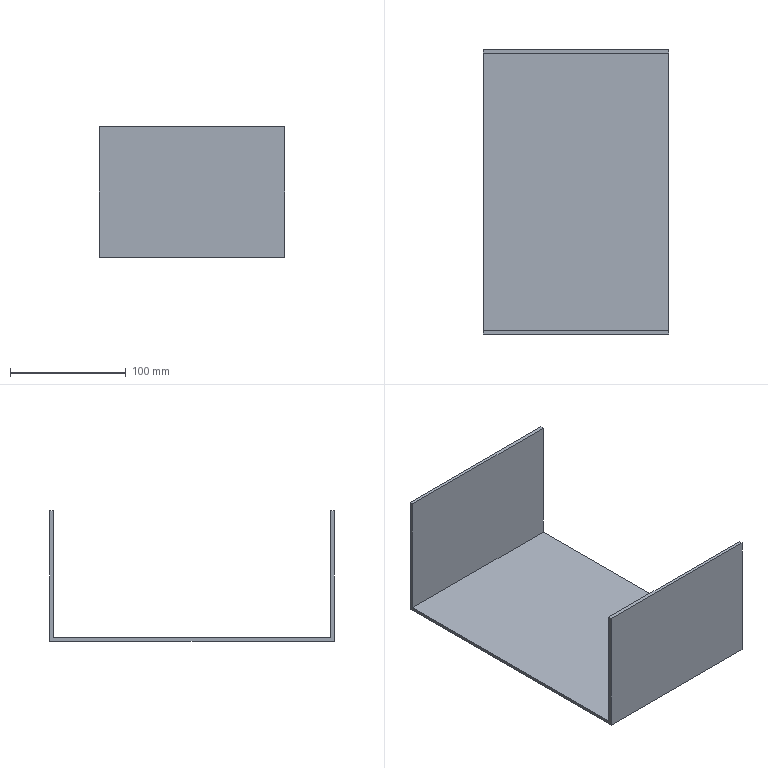Part | SolidWorks | features Extrusion 1, ICE 1 | 1 solid | 10 faces | box 160 x 246 x 113 mm | volume 223680 mm3 | plane 10
STEP:
#1=CARTESIAN_POINT('',(-80.,120.,3.));
#2=VERTEX_POINT('',#1);
#3=CARTESIAN_POINT('',(-80.,-120.,3.));
#4=VERTEX_POINT('',#3);
#5=CARTESIAN_POINT('',(-80.,123.,3.));
#6=DIRECTION('',(0.,-1.,0.));
#7=VECTOR('',#6,1000.);
#8=LINE('',#5,#7);
#9=EDGE_CURVE('',#2,#4,#8,.T.);
#10=ORIENTED_EDGE('',*,*,#9,.T.);
#11=CARTESIAN_POINT('',(80.,-120.,3.));
#12=VERTEX_POINT('',#11);
#13=CARTESIAN_POINT('',(80.,-120.,3.));
#14=DIRECTION('',(-1.,0.,0.));
#15=VECTOR('',#14,1000.);
#16=LINE('',#13,#15);
#17=EDGE_CURVE('',#12,#4,#16,.T.);
#18=ORIENTED_EDGE('',*,*,#17,.F.);
#19=CARTESIAN_POINT('',(80.,120.,3.));
#20=VERTEX_POINT('',#19);
#21=CARTESIAN_POINT('',(80.,123.,3.));
#22=DIRECTION('',(0.,1.,0.));
#23=VECTOR('',#22,1000.);
#24=LINE('',#21,#23);
#25=EDGE_CURVE('',#12,#20,#24,.T.);
#26=ORIENTED_EDGE('',*,*,#25,.T.);
#27=CARTESIAN_POINT('',(-80.,120.,3.));
#28=DIRECTION('',(1.,0.,0.));
#29=VECTOR('',#28,1000.);
#30=LINE('',#27,#29);
#31=EDGE_CURVE('',#2,#20,#30,.T.);
#32=ORIENTED_EDGE('',*,*,#31,.F.);
#33=EDGE_LOOP('',(#10,#18,#26,#32));
#34=FACE_OUTER_BOUND('',#33,.T.);
#35=CARTESIAN_POINT('',(0.,0.,3.));
#36=DIRECTION('',(0.,0.,1.));
#37=DIRECTION('',(1.,0.,0.));
#38=AXIS2_PLACEMENT_3D('',#35,#36,#37);
#39=PLANE('',#38);
#40=ADVANCED_FACE('',(#34),#39,.T.);
#41=CARTESIAN_POINT('',(80.,-123.,0.));
#42=VERTEX_POINT('',#41);
#43=CARTESIAN_POINT('',(80.,123.,0.));
#44=VERTEX_POINT('',#43);
#45=CARTESIAN_POINT('',(80.,123.,0.));
#46=DIRECTION('',(0.,1.,0.));
#47=VECTOR('',#46,1000.);
#48=LINE('',#45,#47);
#49=EDGE_CURVE('',#42,#44,#48,.T.);
#50=ORIENTED_EDGE('',*,*,#49,.T.);
#51=CARTESIAN_POINT('',(80.,123.,113.));
#52=VERTEX_POINT('',#51);
#53=CARTESIAN_POINT('',(80.,123.,3.));
#54=DIRECTION('',(0.,0.,-1.));
#55=VECTOR('',#54,1000.);
#56=LINE('',#53,#55);
#57=EDGE_CURVE('',#52,#44,#56,.T.);
#58=ORIENTED_EDGE('',*,*,#57,.F.);
#59=CARTESIAN_POINT('',(80.,120.,113.));
#60=VERTEX_POINT('',#59);
#61=CARTESIAN_POINT('',(80.,123.,113.));
#62=DIRECTION('',(0.,1.,0.));
#63=VECTOR('',#62,1000.);
#64=LINE('',#61,#63);
#65=EDGE_CURVE('',#60,#52,#64,.T.);
#66=ORIENTED_EDGE('',*,*,#65,.F.);
#67=CARTESIAN_POINT('',(80.,120.,113.));
#68=DIRECTION('',(0.,0.,-1.));
#69=VECTOR('',#68,1000.);
#70=LINE('',#67,#69);
#71=EDGE_CURVE('',#60,#20,#70,.T.);
#72=ORIENTED_EDGE('',*,*,#71,.T.);
#73=ORIENTED_EDGE('',*,*,#25,.F.);
#74=CARTESIAN_POINT('',(80.,-120.,113.));
#75=VERTEX_POINT('',#74);
#76=CARTESIAN_POINT('',(80.,-120.,113.));
#77=DIRECTION('',(0.,0.,-1.));
#78=VECTOR('',#77,1000.);
#79=LINE('',#76,#78);
#80=EDGE_CURVE('',#75,#12,#79,.T.);
#81=ORIENTED_EDGE('',*,*,#80,.F.);
#82=CARTESIAN_POINT('',(80.,-123.,113.));
#83=VERTEX_POINT('',#82);
#84=CARTESIAN_POINT('',(80.,-123.,113.));
#85=DIRECTION('',(0.,1.,0.));
#86=VECTOR('',#85,1000.);
#87=LINE('',#84,#86);
#88=EDGE_CURVE('',#83,#75,#87,.T.);
#89=ORIENTED_EDGE('',*,*,#88,.F.);
#90=CARTESIAN_POINT('',(80.,-123.,3.));
#91=DIRECTION('',(0.,0.,-1.));
#92=VECTOR('',#91,1000.);
#93=LINE('',#90,#92);
#94=EDGE_CURVE('',#83,#42,#93,.T.);
#95=ORIENTED_EDGE('',*,*,#94,.T.);
#96=EDGE_LOOP('',(#50,#58,#66,#72,#73,#81,#89,#95));
#97=FACE_OUTER_BOUND('',#96,.T.);
#98=CARTESIAN_POINT('',(80.,123.,3.));
#99=DIRECTION('',(-1.,0.,0.));
#100=DIRECTION('',(0.,-1.,0.));
#101=AXIS2_PLACEMENT_3D('',#98,#99,#100);
#102=PLANE('',#101);
#103=ADVANCED_FACE('',(#97),#102,.F.);
#104=CARTESIAN_POINT('',(-80.,123.,0.));
#105=VERTEX_POINT('',#104);
#106=CARTESIAN_POINT('',(-80.,123.,0.));
#107=DIRECTION('',(-1.,0.,0.));
#108=VECTOR('',#107,1000.);
#109=LINE('',#106,#108);
#110=EDGE_CURVE('',#44,#105,#109,.T.);
#111=ORIENTED_EDGE('',*,*,#110,.T.);
#112=CARTESIAN_POINT('',(-80.,123.,113.));
#113=VERTEX_POINT('',#112);
#114=CARTESIAN_POINT('',(-80.,123.,3.));
#115=DIRECTION('',(0.,0.,-1.));
#116=VECTOR('',#115,1000.);
#117=LINE('',#114,#116);
#118=EDGE_CURVE('',#113,#105,#117,.T.);
#119=ORIENTED_EDGE('',*,*,#118,.F.);
#120=CARTESIAN_POINT('',(-80.,123.,113.));
#121=DIRECTION('',(-1.,0.,0.));
#122=VECTOR('',#121,1000.);
#123=LINE('',#120,#122);
#124=EDGE_CURVE('',#52,#113,#123,.T.);
#125=ORIENTED_EDGE('',*,*,#124,.F.);
#126=ORIENTED_EDGE('',*,*,#57,.T.);
#127=EDGE_LOOP('',(#111,#119,#125,#126));
#128=FACE_OUTER_BOUND('',#127,.T.);
#129=CARTESIAN_POINT('',(-80.,123.,3.));
#130=DIRECTION('',(0.,-1.,0.));
#131=DIRECTION('',(0.,0.,-1.));
#132=AXIS2_PLACEMENT_3D('',#129,#130,#131);
#133=PLANE('',#132);
#134=ADVANCED_FACE('',(#128),#133,.F.);
#135=CARTESIAN_POINT('',(-80.,-123.,0.));
#136=VERTEX_POINT('',#135);
#137=CARTESIAN_POINT('',(-80.,123.,0.));
#138=DIRECTION('',(0.,-1.,0.));
#139=VECTOR('',#138,1000.);
#140=LINE('',#137,#139);
#141=EDGE_CURVE('',#105,#136,#140,.T.);
#142=ORIENTED_EDGE('',*,*,#141,.T.);
#143=CARTESIAN_POINT('',(-80.,-123.,113.));
#144=VERTEX_POINT('',#143);
#145=CARTESIAN_POINT('',(-80.,-123.,3.));
#146=DIRECTION('',(0.,0.,-1.));
#147=VECTOR('',#146,1000.);
#148=LINE('',#145,#147);
#149=EDGE_CURVE('',#144,#136,#148,.T.);
#150=ORIENTED_EDGE('',*,*,#149,.F.);
#151=CARTESIAN_POINT('',(-80.,-120.,113.));
#152=VERTEX_POINT('',#151);
#153=CARTESIAN_POINT('',(-80.,-123.,113.));
#154=DIRECTION('',(0.,-1.,0.));
#155=VECTOR('',#154,1000.);
#156=LINE('',#153,#155);
#157=EDGE_CURVE('',#152,#144,#156,.T.);
#158=ORIENTED_EDGE('',*,*,#157,.F.);
#159=CARTESIAN_POINT('',(-80.,-120.,113.));
#160=DIRECTION('',(0.,0.,-1.));
#161=VECTOR('',#160,1000.);
#162=LINE('',#159,#161);
#163=EDGE_CURVE('',#152,#4,#162,.T.);
#164=ORIENTED_EDGE('',*,*,#163,.T.);
#165=ORIENTED_EDGE('',*,*,#9,.F.);
#166=CARTESIAN_POINT('',(-80.,120.,113.));
#167=VERTEX_POINT('',#166);
#168=CARTESIAN_POINT('',(-80.,120.,113.));
#169=DIRECTION('',(0.,0.,-1.));
#170=VECTOR('',#169,1000.);
#171=LINE('',#168,#170);
#172=EDGE_CURVE('',#167,#2,#171,.T.);
#173=ORIENTED_EDGE('',*,*,#172,.F.);
#174=CARTESIAN_POINT('',(-80.,123.,113.));
#175=DIRECTION('',(0.,-1.,0.));
#176=VECTOR('',#175,1000.);
#177=LINE('',#174,#176);
#178=EDGE_CURVE('',#113,#167,#177,.T.);
#179=ORIENTED_EDGE('',*,*,#178,.F.);
#180=ORIENTED_EDGE('',*,*,#118,.T.);
#181=EDGE_LOOP('',(#142,#150,#158,#164,#165,#173,#179,#180));
#182=FACE_OUTER_BOUND('',#181,.T.);
#183=CARTESIAN_POINT('',(-80.,123.,3.));
#184=DIRECTION('',(1.,0.,0.));
#185=DIRECTION('',(0.,1.,0.));
#186=AXIS2_PLACEMENT_3D('',#183,#184,#185);
#187=PLANE('',#186);
#188=ADVANCED_FACE('',(#182),#187,.F.);
#189=CARTESIAN_POINT('',(-80.,-123.,0.));
#190=DIRECTION('',(1.,0.,0.));
#191=VECTOR('',#190,1000.);
#192=LINE('',#189,#191);
#193=EDGE_CURVE('',#136,#42,#192,.T.);
#194=ORIENTED_EDGE('',*,*,#193,.T.);
#195=ORIENTED_EDGE('',*,*,#94,.F.);
#196=CARTESIAN_POINT('',(80.,-123.,113.));
#197=DIRECTION('',(1.,0.,0.));
#198=VECTOR('',#197,1000.);
#199=LINE('',#196,#198);
#200=EDGE_CURVE('',#144,#83,#199,.T.);
#201=ORIENTED_EDGE('',*,*,#200,.F.);
#202=ORIENTED_EDGE('',*,*,#149,.T.);
#203=EDGE_LOOP('',(#194,#195,#201,#202));
#204=FACE_OUTER_BOUND('',#203,.T.);
#205=CARTESIAN_POINT('',(-80.,-123.,3.));
#206=DIRECTION('',(0.,1.,0.));
#207=DIRECTION('',(0.,0.,1.));
#208=AXIS2_PLACEMENT_3D('',#205,#206,#207);
#209=PLANE('',#208);
#210=ADVANCED_FACE('',(#204),#209,.F.);
#211=ORIENTED_EDGE('',*,*,#49,.F.);
#212=ORIENTED_EDGE('',*,*,#193,.F.);
#213=ORIENTED_EDGE('',*,*,#141,.F.);
#214=ORIENTED_EDGE('',*,*,#110,.F.);
#215=EDGE_LOOP('',(#211,#212,#213,#214));
#216=FACE_OUTER_BOUND('',#215,.T.);
#217=CARTESIAN_POINT('',(0.,0.,0.));
#218=DIRECTION('',(0.,0.,1.));
#219=DIRECTION('',(1.,0.,0.));
#220=AXIS2_PLACEMENT_3D('',#217,#218,#219);
#221=PLANE('',#220);
#222=ADVANCED_FACE('',(#216),#221,.F.);
#223=ORIENTED_EDGE('',*,*,#31,.T.);
#224=ORIENTED_EDGE('',*,*,#71,.F.);
#225=CARTESIAN_POINT('',(-80.,120.,113.));
#226=DIRECTION('',(1.,0.,0.));
#227=VECTOR('',#226,1000.);
#228=LINE('',#225,#227);
#229=EDGE_CURVE('',#167,#60,#228,.T.);
#230=ORIENTED_EDGE('',*,*,#229,.F.);
#231=ORIENTED_EDGE('',*,*,#172,.T.);
#232=EDGE_LOOP('',(#223,#224,#230,#231));
#233=FACE_OUTER_BOUND('',#232,.T.);
#234=CARTESIAN_POINT('',(-80.,120.,113.));
#235=DIRECTION('',(0.,1.,0.));
#236=DIRECTION('',(-1.,0.,0.));
#237=AXIS2_PLACEMENT_3D('',#234,#235,#236);
#238=PLANE('',#237);
#239=ADVANCED_FACE('',(#233),#238,.F.);
#240=ORIENTED_EDGE('',*,*,#178,.T.);
#241=ORIENTED_EDGE('',*,*,#229,.T.);
#242=ORIENTED_EDGE('',*,*,#65,.T.);
#243=ORIENTED_EDGE('',*,*,#124,.T.);
#244=EDGE_LOOP('',(#240,#241,#242,#243));
#245=FACE_OUTER_BOUND('',#244,.T.);
#246=CARTESIAN_POINT('',(0.,0.,113.));
#247=DIRECTION('',(0.,0.,1.));
#248=DIRECTION('',(1.,0.,0.));
#249=AXIS2_PLACEMENT_3D('',#246,#247,#248);
#250=PLANE('',#249);
#251=ADVANCED_FACE('',(#245),#250,.T.);
#252=ORIENTED_EDGE('',*,*,#17,.T.);
#253=ORIENTED_EDGE('',*,*,#163,.F.);
#254=CARTESIAN_POINT('',(80.,-120.,113.));
#255=DIRECTION('',(-1.,0.,0.));
#256=VECTOR('',#255,1000.);
#257=LINE('',#254,#256);
#258=EDGE_CURVE('',#75,#152,#257,.T.);
#259=ORIENTED_EDGE('',*,*,#258,.F.);
#260=ORIENTED_EDGE('',*,*,#80,.T.);
#261=EDGE_LOOP('',(#252,#253,#259,#260));
#262=FACE_OUTER_BOUND('',#261,.T.);
#263=CARTESIAN_POINT('',(80.,-120.,113.));
#264=DIRECTION('',(0.,-1.,0.));
#265=DIRECTION('',(1.,0.,0.));
#266=AXIS2_PLACEMENT_3D('',#263,#264,#265);
#267=PLANE('',#266);
#268=ADVANCED_FACE('',(#262),#267,.F.);
#269=ORIENTED_EDGE('',*,*,#88,.T.);
#270=ORIENTED_EDGE('',*,*,#258,.T.);
#271=ORIENTED_EDGE('',*,*,#157,.T.);
#272=ORIENTED_EDGE('',*,*,#200,.T.);
#273=EDGE_LOOP('',(#269,#270,#271,#272));
#274=FACE_OUTER_BOUND('',#273,.T.);
#275=CARTESIAN_POINT('',(0.,0.,113.));
#276=DIRECTION('',(0.,0.,1.));
#277=DIRECTION('',(1.,0.,0.));
#278=AXIS2_PLACEMENT_3D('',#275,#276,#277);
#279=PLANE('',#278);
#280=ADVANCED_FACE('',(#274),#279,.T.);
#281=CLOSED_SHELL('',(#40,#103,#134,#188,#210,#222,#239,#251,#268,#280));
#282=MANIFOLD_SOLID_BREP('',#281);
#283=CARTESIAN_POINT('',(0.,0.,0.));
#284=DIRECTION('',(0.,0.,1.));
#285=DIRECTION('',(1.,0.,0.));
#286=AXIS2_PLACEMENT_3D('',#283,#284,#285);
#287=(LENGTH_UNIT()NAMED_UNIT(*)SI_UNIT(.MILLI.,.METRE.));
#288=UNCERTAINTY_MEASURE_WITH_UNIT(LENGTH_MEASURE(0.00001),#287,'','');
#289=(NAMED_UNIT(*)PLANE_ANGLE_UNIT()SI_UNIT($,.RADIAN.));
#290=(NAMED_UNIT(*)SI_UNIT($,.STERADIAN.)SOLID_ANGLE_UNIT());
#291=(GEOMETRIC_REPRESENTATION_CONTEXT(3)GLOBAL_UNCERTAINTY_ASSIGNED_CONTEXT((#288))GLOBAL_UNIT_ASSIGNED_CONTEXT((#287,#289,#290))REPRESENTATION_CONTEXT('',''));
#292=ADVANCED_BREP_SHAPE_REPRESENTATION('',(#282,#286),#291);